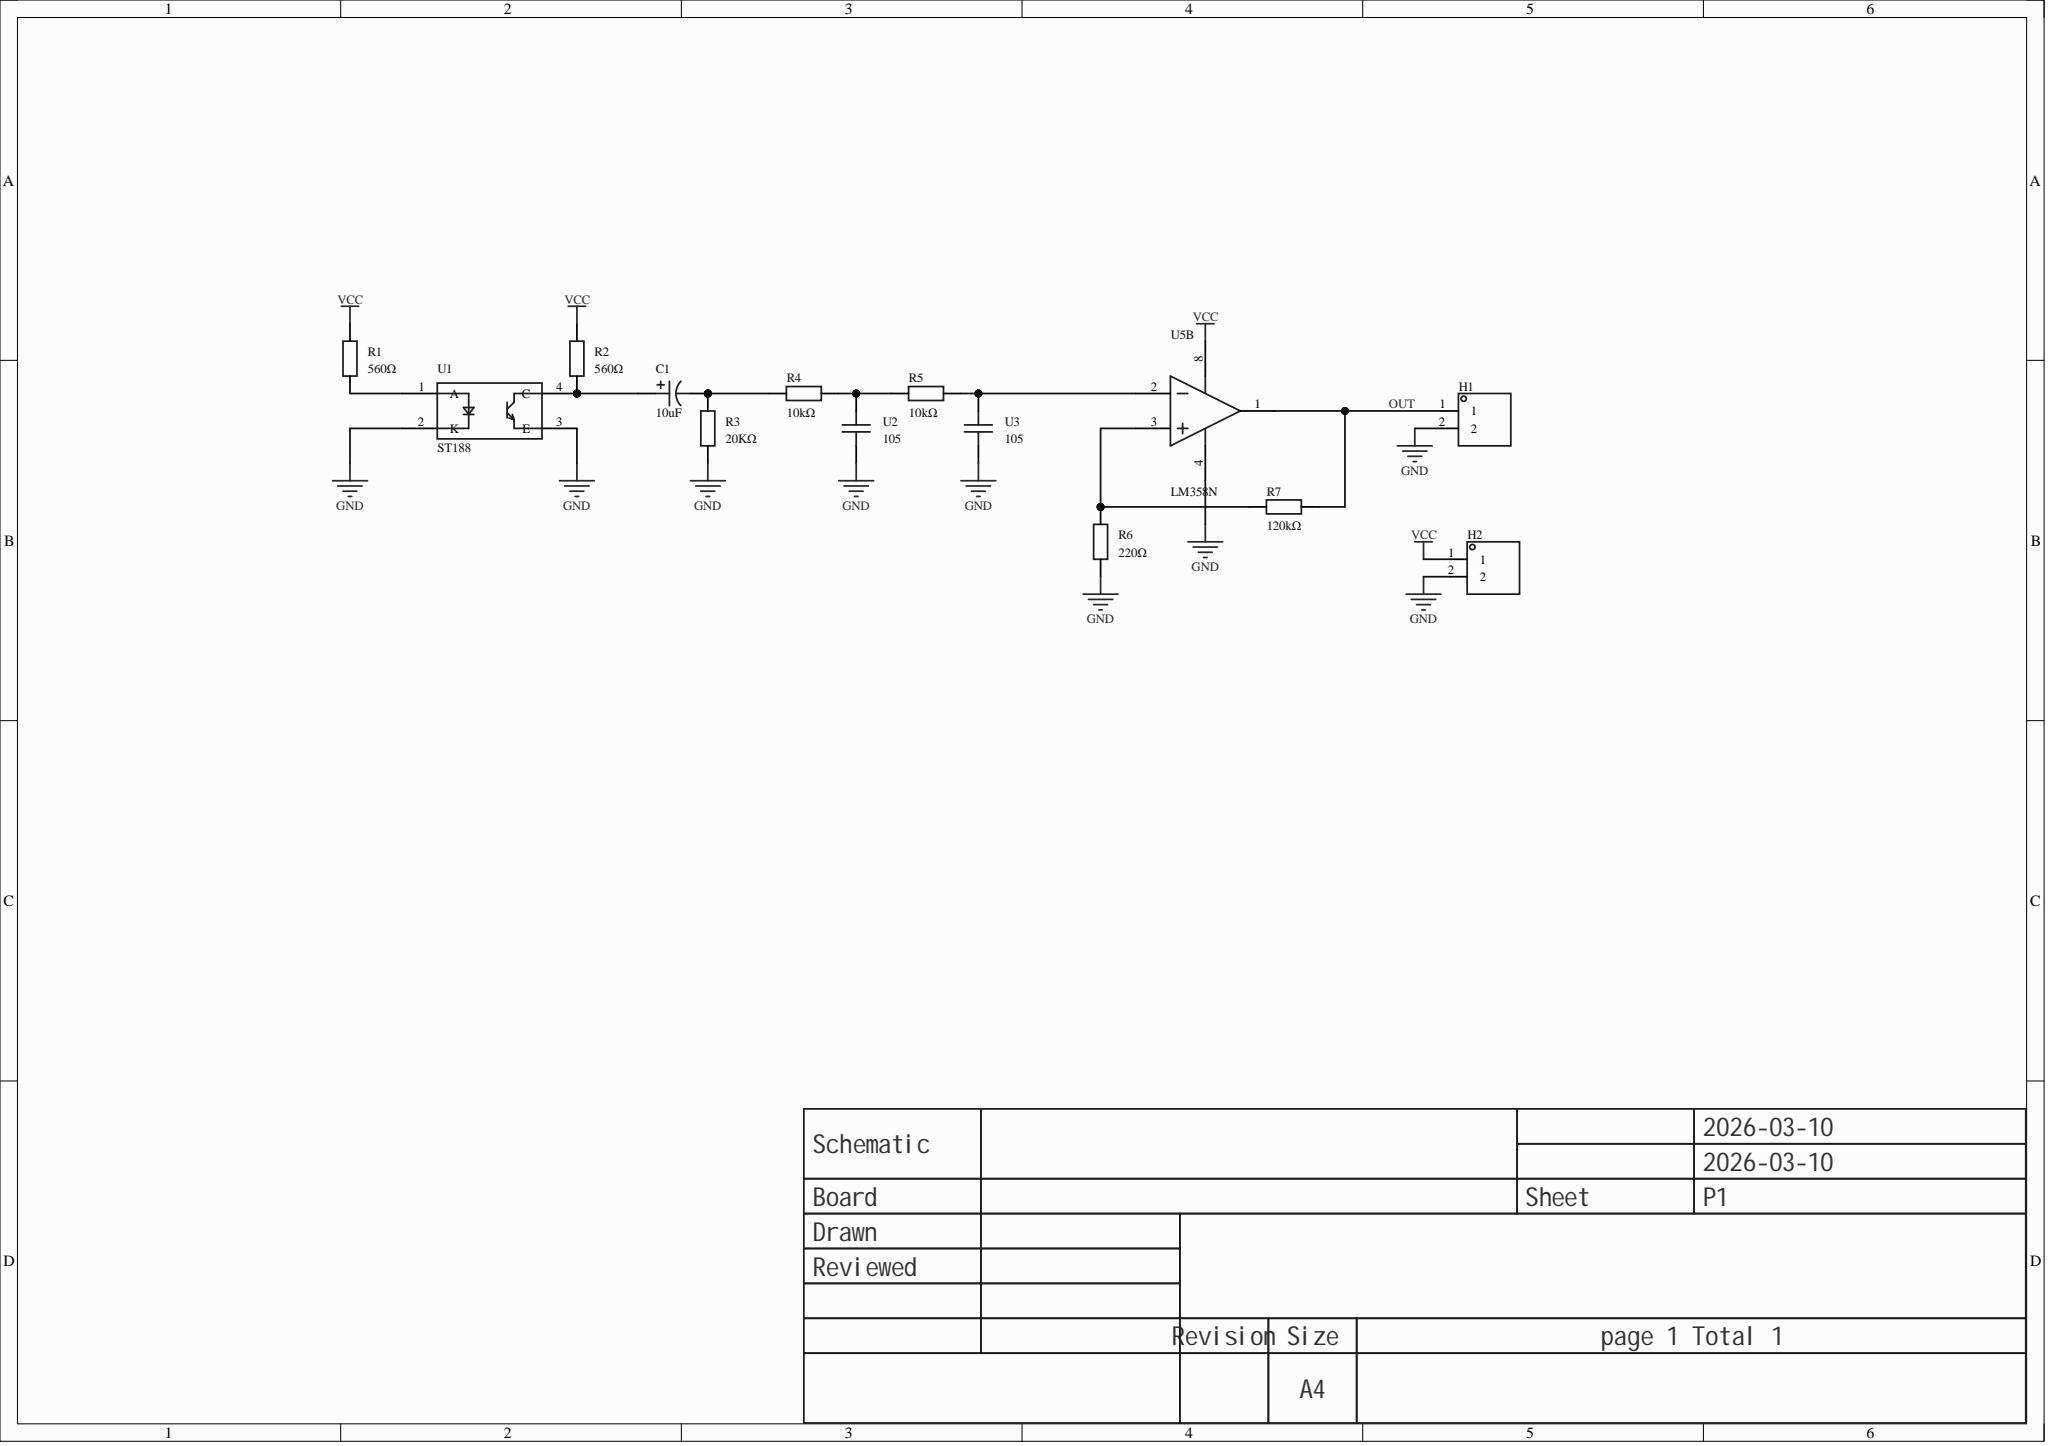Circuit board | Altium Designer | 14 parts | 9 nets
Bill of materials:
Comment,Description,Designator,Footprint,LibRef,Quantity
"10uF","Capacitance:10uF; Tolerance:±20%; Rated voltage:50V; Ripple current:120mA@100KHz; ESR:1.6Ω;","C1","CAP-TH_BD5.0-P2.00-D0.8-FD-10UF50VC110GL","10UF50VC110GL","1"
"","","H1, H2","HDR-TH_2P-P2.54-V-M-1","HDR-M_2.54_1x2P","2"
"560Ω","","R1, R2","Res_1/8W","Res_AXIAL-1/8W","2"
"20KΩ","","R3","Res_1/8W","Res_AXIAL-1/8W","1"
"10kΩ","","R4, R5","Res_1/8W","Res_AXIAL-1/8W","2"
"220Ω","","R6","Res_1/8W","Res_AXIAL-1/8W","1"
"120kΩ","","R7","Res_1/8W","Res_AXIAL-1/8W","1"
"ST188","","U1","OPTO-TH_ST188","ST188","1"
"105","","U2, U3","CAP-TH_L5.0-W2.5-P5.00-D1.0","100nF","2"
"LM358N","Number of amplifiers: dual; Gain bandwidth product (GBP): 1MHz; Slew rate (SR): 0.6V/us;","U5","DIP-8_L9.2-W6.4-P2.54-LS7.6-BL","LM358N_C84858","1"
Netlist (Protel format):
[
C1
CAP-TH_BD5.0-P2.00-D0.8-FD-10UF50VC110GL
10uF



]
[
H1
HDR-TH_2P-P2.54-V-M-1




]
[
H2
HDR-TH_2P-P2.54-V-M-1




]
[
R1
Res_1/8W
560Ω



]
[
R2
Res_1/8W
560Ω



]
[
R3
Res_1/8W
20KΩ



]
[
R4
Res_1/8W
10kΩ



]
[
R5
Res_1/8W
10kΩ



]
[
R6
Res_1/8W
220Ω



]
[
R7
Res_1/8W
120kΩ



]
[
U1
OPTO-TH_ST188
ST188



]
[
U2
CAP-TH_L5.0-W2.5-P5.00-D1.0
105



]
[
U3
CAP-TH_L5.0-W2.5-P5.00-D1.0
105



]
[
U5
DIP-8_L9.2-W6.4-P2.54-LS7.6-BL
LM358N



]
(
VCC
H2-1
R1-2
R2-2
U5-8
)
(
OUT
H1-1
R7-2
U5-1
)
(
NetR6_2
R6-2
R7-1
U5-3
)
(
NetR5_2
R5-2
U3-1
U5-2
)
(
NetR4_2
R4-2
R5-1
U2-1
)
(
NetR1_1
R1-1
U1-1
)
(
NetC1_2
C1-2
R3-2
R4-1
)
(
NetC1_1
C1-1
R2-1
U1-4
)
(
GND
H1-2
H2-2
R3-1
R6-1
U1-2
U1-3
U2-2
U3-2
U5-4
)